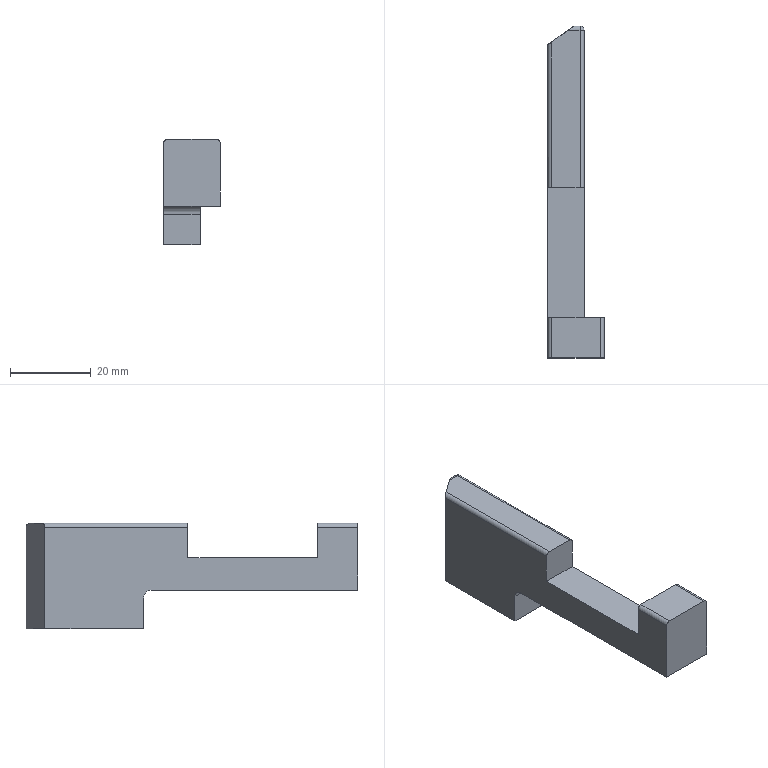Part | NX | features DIE-37 2 | 1 solid | 22 faces | box 14 x 82 x 26 mm | volume 12622 mm3 | plane 14 | cylinder 7 | sphere 1 | commonest cylinder face diameters 2 x6 4 x1
STEP:
#1=CARTESIAN_POINT('',(2459.569,-953.622,868.716));
#2=VERTEX_POINT('',#1);
#3=CARTESIAN_POINT('',(2459.569,-1004.622,868.716));
#4=VERTEX_POINT('',#3);
#5=CARTESIAN_POINT('',(2459.569,-923.622,868.716));
#6=DIRECTION('',(0.,-1.,0.));
#7=VECTOR('',#6,1000.);
#8=LINE('',#5,#7);
#9=EDGE_CURVE('',#2,#4,#8,.T.);
#10=ORIENTED_EDGE('',*,*,#9,.F.);
#11=CARTESIAN_POINT('',(2468.569,-953.622,868.716));
#12=VERTEX_POINT('',#11);
#13=CARTESIAN_POINT('',(2465.569,-953.622,868.716));
#14=DIRECTION('',(1.,0.,0.));
#15=VECTOR('',#14,1000.);
#16=LINE('',#13,#15);
#17=EDGE_CURVE('',#2,#12,#16,.T.);
#18=ORIENTED_EDGE('',*,*,#17,.T.);
#19=CARTESIAN_POINT('',(2468.569,-994.622,868.716));
#20=VERTEX_POINT('',#19);
#21=CARTESIAN_POINT('',(2468.569,-923.622,868.716));
#22=DIRECTION('',(0.,1.,0.));
#23=VECTOR('',#22,1000.);
#24=LINE('',#21,#23);
#25=EDGE_CURVE('',#20,#12,#24,.T.);
#26=ORIENTED_EDGE('',*,*,#25,.F.);
#27=CARTESIAN_POINT('',(2473.569,-994.622,868.716));
#28=VERTEX_POINT('',#27);
#29=CARTESIAN_POINT('',(2465.569,-994.622,868.716));
#30=DIRECTION('',(-1.,0.,0.));
#31=VECTOR('',#30,1000.);
#32=LINE('',#29,#31);
#33=EDGE_CURVE('',#28,#20,#32,.T.);
#34=ORIENTED_EDGE('',*,*,#33,.F.);
#35=CARTESIAN_POINT('',(2473.569,-1004.622,868.716));
#36=VERTEX_POINT('',#35);
#37=CARTESIAN_POINT('',(2473.569,-923.622,868.716));
#38=DIRECTION('',(0.,1.,0.));
#39=VECTOR('',#38,1000.);
#40=LINE('',#37,#39);
#41=EDGE_CURVE('',#36,#28,#40,.T.);
#42=ORIENTED_EDGE('',*,*,#41,.F.);
#43=CARTESIAN_POINT('',(2691.569,-1004.622,868.716));
#44=DIRECTION('',(1.,0.,0.));
#45=VECTOR('',#44,1000.);
#46=LINE('',#43,#45);
#47=EDGE_CURVE('',#4,#36,#46,.T.);
#48=ORIENTED_EDGE('',*,*,#47,.F.);
#49=EDGE_LOOP('',(#10,#18,#26,#34,#42,#48));
#50=FACE_BOUND('',#49,.T.);
#51=CARTESIAN_POINT('',(2465.569,-923.622,868.716));
#52=DIRECTION('',(0.,0.,-1.));
#53=DIRECTION('',(1.,0.,0.));
#54=AXIS2_PLACEMENT_3D('',#51,#52,#53);
#55=PLANE('',#54);
#56=ADVANCED_FACE('',(#50),#55,.T.);
#57=CARTESIAN_POINT('',(2468.569,-994.622,876.716));
#58=VERTEX_POINT('',#57);
#59=CARTESIAN_POINT('',(2468.569,-994.622,868.716));
#60=DIRECTION('',(0.,0.,-1.));
#61=VECTOR('',#60,1000.);
#62=LINE('',#59,#61);
#63=EDGE_CURVE('',#58,#20,#62,.T.);
#64=ORIENTED_EDGE('',*,*,#63,.F.);
#65=CARTESIAN_POINT('',(2459.569,-994.622,876.716));
#66=VERTEX_POINT('',#65);
#67=CARTESIAN_POINT('',(2691.569,-994.622,876.716));
#68=DIRECTION('',(-1.,0.,0.));
#69=VECTOR('',#68,1000.);
#70=LINE('',#67,#69);
#71=EDGE_CURVE('',#58,#66,#70,.T.);
#72=ORIENTED_EDGE('',*,*,#71,.T.);
#73=CARTESIAN_POINT('',(2459.569,-994.622,884.216));
#74=VERTEX_POINT('',#73);
#75=CARTESIAN_POINT('',(2459.569,-994.622,868.716));
#76=DIRECTION('',(0.,0.,1.));
#77=VECTOR('',#76,1000.);
#78=LINE('',#75,#77);
#79=EDGE_CURVE('',#66,#74,#78,.T.);
#80=ORIENTED_EDGE('',*,*,#79,.T.);
#81=CARTESIAN_POINT('',(2460.569,-994.622,885.216));
#82=VERTEX_POINT('',#81);
#83=CARTESIAN_POINT('',(2460.569,-994.622,884.216));
#84=DIRECTION('',(0.,1.,0.));
#85=DIRECTION('',(0.,0.,-1.));
#86=AXIS2_PLACEMENT_3D('',#83,#84,#85);
#87=CIRCLE('',#86,1.);
#88=EDGE_CURVE('',#74,#82,#87,.T.);
#89=ORIENTED_EDGE('',*,*,#88,.T.);
#90=CARTESIAN_POINT('',(2472.569,-994.622,885.216));
#91=VERTEX_POINT('',#90);
#92=CARTESIAN_POINT('',(2691.569,-994.622,885.216));
#93=DIRECTION('',(-1.,0.,0.));
#94=VECTOR('',#93,1000.);
#95=LINE('',#92,#94);
#96=EDGE_CURVE('',#91,#82,#95,.T.);
#97=ORIENTED_EDGE('',*,*,#96,.F.);
#98=CARTESIAN_POINT('',(2473.569,-994.622,884.216));
#99=VERTEX_POINT('',#98);
#100=CARTESIAN_POINT('',(2472.569,-994.622,884.216));
#101=DIRECTION('',(0.,1.,0.));
#102=DIRECTION('',(0.,0.,-1.));
#103=AXIS2_PLACEMENT_3D('',#100,#101,#102);
#104=CIRCLE('',#103,1.);
#105=EDGE_CURVE('',#91,#99,#104,.T.);
#106=ORIENTED_EDGE('',*,*,#105,.T.);
#107=CARTESIAN_POINT('',(2473.569,-994.622,803.716));
#108=DIRECTION('',(0.,0.,1.));
#109=VECTOR('',#108,1000.);
#110=LINE('',#107,#109);
#111=EDGE_CURVE('',#28,#99,#110,.T.);
#112=ORIENTED_EDGE('',*,*,#111,.F.);
#113=ORIENTED_EDGE('',*,*,#33,.T.);
#114=EDGE_LOOP('',(#64,#72,#80,#89,#97,#106,#112,#113));
#115=FACE_BOUND('',#114,.T.);
#116=CARTESIAN_POINT('',(2691.569,-994.622,803.716));
#117=DIRECTION('',(0.,-1.,0.));
#118=DIRECTION('',(0.,0.,-1.));
#119=AXIS2_PLACEMENT_3D('',#116,#117,#118);
#120=PLANE('',#119);
#121=ADVANCED_FACE('',(#115),#120,.F.);
#122=ORIENTED_EDGE('',*,*,#96,.T.);
#123=CARTESIAN_POINT('',(2460.569,-1004.622,885.216));
#124=VERTEX_POINT('',#123);
#125=CARTESIAN_POINT('',(2460.569,-913.622,885.216));
#126=DIRECTION('',(0.,-1.,0.));
#127=VECTOR('',#126,1000.);
#128=LINE('',#125,#127);
#129=EDGE_CURVE('',#82,#124,#128,.T.);
#130=ORIENTED_EDGE('',*,*,#129,.T.);
#131=CARTESIAN_POINT('',(2472.569,-1004.622,885.216));
#132=VERTEX_POINT('',#131);
#133=CARTESIAN_POINT('',(2691.569,-1004.622,885.216));
#134=DIRECTION('',(-1.,0.,0.));
#135=VECTOR('',#134,1000.);
#136=LINE('',#133,#135);
#137=EDGE_CURVE('',#132,#124,#136,.T.);
#138=ORIENTED_EDGE('',*,*,#137,.F.);
#139=CARTESIAN_POINT('',(2472.569,-913.622,885.216));
#140=DIRECTION('',(0.,1.,0.));
#141=VECTOR('',#140,1000.);
#142=LINE('',#139,#141);
#143=EDGE_CURVE('',#132,#91,#142,.T.);
#144=ORIENTED_EDGE('',*,*,#143,.T.);
#145=EDGE_LOOP('',(#122,#130,#138,#144));
#146=FACE_BOUND('',#145,.T.);
#147=CARTESIAN_POINT('',(2465.569,-913.622,885.216));
#148=DIRECTION('',(0.,0.,1.));
#149=DIRECTION('',(-1.,0.,0.));
#150=AXIS2_PLACEMENT_3D('',#147,#148,#149);
#151=PLANE('',#150);
#152=ADVANCED_FACE('',(#146),#151,.T.);
#153=ORIENTED_EDGE('',*,*,#105,.F.);
#154=ORIENTED_EDGE('',*,*,#143,.F.);
#155=CARTESIAN_POINT('',(2473.569,-1004.622,884.216));
#156=VERTEX_POINT('',#155);
#157=CARTESIAN_POINT('',(2472.569,-1004.622,884.216));
#158=DIRECTION('',(0.,-1.,0.));
#159=DIRECTION('',(0.,0.,-1.));
#160=AXIS2_PLACEMENT_3D('',#157,#158,#159);
#161=CIRCLE('',#160,1.);
#162=EDGE_CURVE('',#156,#132,#161,.T.);
#163=ORIENTED_EDGE('',*,*,#162,.F.);
#164=CARTESIAN_POINT('',(2473.569,-913.622,884.216));
#165=DIRECTION('',(0.,-1.,0.));
#166=VECTOR('',#165,1000.);
#167=LINE('',#164,#166);
#168=EDGE_CURVE('',#99,#156,#167,.T.);
#169=ORIENTED_EDGE('',*,*,#168,.F.);
#170=EDGE_LOOP('',(#153,#154,#163,#169));
#171=FACE_BOUND('',#170,.T.);
#172=CARTESIAN_POINT('',(2472.569,-913.622,884.216));
#173=DIRECTION('',(0.,-1.,0.));
#174=DIRECTION('',(0.,0.,1.));
#175=AXIS2_PLACEMENT_3D('',#172,#173,#174);
#176=CYLINDRICAL_SURFACE('',#175,1.);
#177=ADVANCED_FACE('',(#171),#176,.T.);
#178=CARTESIAN_POINT('',(2459.569,-1004.622,884.216));
#179=VERTEX_POINT('',#178);
#180=CARTESIAN_POINT('',(2460.569,-1004.622,884.216));
#181=DIRECTION('',(0.,-1.,0.));
#182=DIRECTION('',(0.,0.,-1.));
#183=AXIS2_PLACEMENT_3D('',#180,#181,#182);
#184=CIRCLE('',#183,1.);
#185=EDGE_CURVE('',#124,#179,#184,.T.);
#186=ORIENTED_EDGE('',*,*,#185,.F.);
#187=ORIENTED_EDGE('',*,*,#129,.F.);
#188=ORIENTED_EDGE('',*,*,#88,.F.);
#189=CARTESIAN_POINT('',(2459.569,-913.622,884.216));
#190=DIRECTION('',(0.,1.,0.));
#191=VECTOR('',#190,1000.);
#192=LINE('',#189,#191);
#193=EDGE_CURVE('',#179,#74,#192,.T.);
#194=ORIENTED_EDGE('',*,*,#193,.F.);
#195=EDGE_LOOP('',(#186,#187,#188,#194));
#196=FACE_BOUND('',#195,.T.);
#197=CARTESIAN_POINT('',(2460.569,-913.622,884.216));
#198=DIRECTION('',(0.,1.,0.));
#199=DIRECTION('',(0.,0.,-1.));
#200=AXIS2_PLACEMENT_3D('',#197,#198,#199);
#201=CYLINDRICAL_SURFACE('',#200,1.);
#202=ADVANCED_FACE('',(#196),#201,.T.);
#203=ORIENTED_EDGE('',*,*,#137,.T.);
#204=ORIENTED_EDGE('',*,*,#185,.T.);
#205=CARTESIAN_POINT('',(2459.569,-1004.622,868.716));
#206=DIRECTION('',(0.,0.,1.));
#207=VECTOR('',#206,1000.);
#208=LINE('',#205,#207);
#209=EDGE_CURVE('',#4,#179,#208,.T.);
#210=ORIENTED_EDGE('',*,*,#209,.F.);
#211=ORIENTED_EDGE('',*,*,#47,.T.);
#212=CARTESIAN_POINT('',(2473.569,-1004.622,803.716));
#213=DIRECTION('',(0.,0.,1.));
#214=VECTOR('',#213,1000.);
#215=LINE('',#212,#214);
#216=EDGE_CURVE('',#36,#156,#215,.T.);
#217=ORIENTED_EDGE('',*,*,#216,.T.);
#218=ORIENTED_EDGE('',*,*,#162,.T.);
#219=EDGE_LOOP('',(#203,#204,#210,#211,#217,#218));
#220=FACE_BOUND('',#219,.T.);
#221=CARTESIAN_POINT('',(2691.569,-1004.622,803.716));
#222=DIRECTION('',(0.,-1.,0.));
#223=DIRECTION('',(0.,0.,-1.));
#224=AXIS2_PLACEMENT_3D('',#221,#222,#223);
#225=PLANE('',#224);
#226=ADVANCED_FACE('',(#220),#225,.T.);
#227=ORIENTED_EDGE('',*,*,#79,.F.);
#228=CARTESIAN_POINT('',(2459.569,-962.622,876.716));
#229=VERTEX_POINT('',#228);
#230=CARTESIAN_POINT('',(2459.569,-923.622,876.716));
#231=DIRECTION('',(0.,1.,0.));
#232=VECTOR('',#231,1000.);
#233=LINE('',#230,#232);
#234=EDGE_CURVE('',#66,#229,#233,.T.);
#235=ORIENTED_EDGE('',*,*,#234,.T.);
#236=CARTESIAN_POINT('',(2459.569,-962.622,884.216));
#237=VERTEX_POINT('',#236);
#238=CARTESIAN_POINT('',(2459.569,-962.622,868.716));
#239=DIRECTION('',(0.,0.,-1.));
#240=VECTOR('',#239,1000.);
#241=LINE('',#238,#240);
#242=EDGE_CURVE('',#237,#229,#241,.T.);
#243=ORIENTED_EDGE('',*,*,#242,.F.);
#244=CARTESIAN_POINT('',(2459.569,-927.265,884.216));
#245=VERTEX_POINT('',#244);
#246=CARTESIAN_POINT('',(2459.569,-923.622,884.216));
#247=DIRECTION('',(0.,1.,0.));
#248=VECTOR('',#247,1000.);
#249=LINE('',#246,#248);
#250=EDGE_CURVE('',#237,#245,#249,.T.);
#251=ORIENTED_EDGE('',*,*,#250,.T.);
#252=CARTESIAN_POINT('',(2459.569,-927.265,859.216));
#253=VERTEX_POINT('',#252);
#254=CARTESIAN_POINT('',(2459.569,-927.265,868.716));
#255=DIRECTION('',(0.,0.,-1.));
#256=VECTOR('',#255,1000.);
#257=LINE('',#254,#256);
#258=EDGE_CURVE('',#245,#253,#257,.T.);
#259=ORIENTED_EDGE('',*,*,#258,.T.);
#260=CARTESIAN_POINT('',(2459.569,-951.622,859.216));
#261=VERTEX_POINT('',#260);
#262=CARTESIAN_POINT('',(2459.569,-923.622,859.216));
#263=DIRECTION('',(0.,-1.,0.));
#264=VECTOR('',#263,1000.);
#265=LINE('',#262,#264);
#266=EDGE_CURVE('',#253,#261,#265,.T.);
#267=ORIENTED_EDGE('',*,*,#266,.T.);
#268=CARTESIAN_POINT('',(2459.569,-951.622,866.716));
#269=VERTEX_POINT('',#268);
#270=CARTESIAN_POINT('',(2459.569,-951.622,868.716));
#271=DIRECTION('',(0.,0.,1.));
#272=VECTOR('',#271,1000.);
#273=LINE('',#270,#272);
#274=EDGE_CURVE('',#261,#269,#273,.T.);
#275=ORIENTED_EDGE('',*,*,#274,.T.);
#276=CARTESIAN_POINT('',(2459.569,-953.622,866.716));
#277=DIRECTION('',(-1.,0.,0.));
#278=DIRECTION('',(0.,0.,1.));
#279=AXIS2_PLACEMENT_3D('',#276,#277,#278);
#280=CIRCLE('',#279,2.);
#281=EDGE_CURVE('',#269,#2,#280,.F.);
#282=ORIENTED_EDGE('',*,*,#281,.T.);
#283=ORIENTED_EDGE('',*,*,#9,.T.);
#284=ORIENTED_EDGE('',*,*,#209,.T.);
#285=ORIENTED_EDGE('',*,*,#193,.T.);
#286=EDGE_LOOP('',(#227,#235,#243,#251,#259,#267,#275,#282,#283,#284,#285));
#287=FACE_BOUND('',#286,.T.);
#288=CARTESIAN_POINT('',(2459.569,-923.622,868.716));
#289=DIRECTION('',(-1.,0.,0.));
#290=DIRECTION('',(0.,0.,-1.));
#291=AXIS2_PLACEMENT_3D('',#288,#289,#290);
#292=PLANE('',#291);
#293=ADVANCED_FACE('',(#287),#292,.T.);
#294=ORIENTED_EDGE('',*,*,#41,.T.);
#295=ORIENTED_EDGE('',*,*,#111,.T.);
#296=ORIENTED_EDGE('',*,*,#168,.T.);
#297=ORIENTED_EDGE('',*,*,#216,.F.);
#298=EDGE_LOOP('',(#294,#295,#296,#297));
#299=FACE_BOUND('',#298,.T.);
#300=CARTESIAN_POINT('',(2473.569,-923.622,868.716));
#301=DIRECTION('',(1.,0.,0.));
#302=DIRECTION('',(0.,0.,1.));
#303=AXIS2_PLACEMENT_3D('',#300,#301,#302);
#304=PLANE('',#303);
#305=ADVANCED_FACE('',(#299),#304,.T.);
#306=ORIENTED_EDGE('',*,*,#25,.T.);
#307=CARTESIAN_POINT('',(2468.569,-951.622,866.716));
#308=VERTEX_POINT('',#307);
#309=CARTESIAN_POINT('',(2468.569,-953.622,866.716));
#310=DIRECTION('',(1.,0.,0.));
#311=DIRECTION('',(0.,0.,-1.));
#312=AXIS2_PLACEMENT_3D('',#309,#310,#311);
#313=CIRCLE('',#312,2.);
#314=EDGE_CURVE('',#12,#308,#313,.F.);
#315=ORIENTED_EDGE('',*,*,#314,.T.);
#316=CARTESIAN_POINT('',(2468.569,-951.622,859.216));
#317=VERTEX_POINT('',#316);
#318=CARTESIAN_POINT('',(2468.569,-951.622,868.716));
#319=DIRECTION('',(0.,0.,-1.));
#320=VECTOR('',#319,1000.);
#321=LINE('',#318,#320);
#322=EDGE_CURVE('',#317,#308,#321,.F.);
#323=ORIENTED_EDGE('',*,*,#322,.F.);
#324=CARTESIAN_POINT('',(2468.569,-923.622,859.216));
#325=VERTEX_POINT('',#324);
#326=CARTESIAN_POINT('',(2468.569,-923.622,859.216));
#327=DIRECTION('',(0.,1.,0.));
#328=VECTOR('',#327,1000.);
#329=LINE('',#326,#328);
#330=EDGE_CURVE('',#317,#325,#329,.T.);
#331=ORIENTED_EDGE('',*,*,#330,.T.);
#332=CARTESIAN_POINT('',(2468.569,-923.622,884.216));
#333=VERTEX_POINT('',#332);
#334=CARTESIAN_POINT('',(2468.569,-923.622,868.716));
#335=DIRECTION('',(0.,0.,1.));
#336=VECTOR('',#335,1000.);
#337=LINE('',#334,#336);
#338=EDGE_CURVE('',#325,#333,#337,.T.);
#339=ORIENTED_EDGE('',*,*,#338,.T.);
#340=CARTESIAN_POINT('',(2468.569,-962.622,884.216));
#341=VERTEX_POINT('',#340);
#342=CARTESIAN_POINT('',(2468.569,-923.622,884.216));
#343=DIRECTION('',(0.,-1.,0.));
#344=VECTOR('',#343,1000.);
#345=LINE('',#342,#344);
#346=EDGE_CURVE('',#333,#341,#345,.T.);
#347=ORIENTED_EDGE('',*,*,#346,.T.);
#348=CARTESIAN_POINT('',(2468.569,-962.622,876.716));
#349=VERTEX_POINT('',#348);
#350=CARTESIAN_POINT('',(2468.569,-962.622,868.716));
#351=DIRECTION('',(0.,0.,1.));
#352=VECTOR('',#351,1000.);
#353=LINE('',#350,#352);
#354=EDGE_CURVE('',#349,#341,#353,.T.);
#355=ORIENTED_EDGE('',*,*,#354,.F.);
#356=CARTESIAN_POINT('',(2468.569,-923.622,876.716));
#357=DIRECTION('',(0.,-1.,0.));
#358=VECTOR('',#357,1000.);
#359=LINE('',#356,#358);
#360=EDGE_CURVE('',#349,#58,#359,.T.);
#361=ORIENTED_EDGE('',*,*,#360,.T.);
#362=ORIENTED_EDGE('',*,*,#63,.T.);
#363=EDGE_LOOP('',(#306,#315,#323,#331,#339,#347,#355,#361,#362));
#364=FACE_BOUND('',#363,.T.);
#365=CARTESIAN_POINT('',(2468.569,-923.622,868.716));
#366=DIRECTION('',(1.,0.,0.));
#367=DIRECTION('',(0.,0.,1.));
#368=AXIS2_PLACEMENT_3D('',#365,#366,#367);
#369=PLANE('',#368);
#370=ADVANCED_FACE('',(#364),#369,.T.);
#371=ORIENTED_EDGE('',*,*,#234,.F.);
#372=ORIENTED_EDGE('',*,*,#71,.F.);
#373=ORIENTED_EDGE('',*,*,#360,.F.);
#374=CARTESIAN_POINT('',(2463.569,-962.622,876.716));
#375=DIRECTION('',(-1.,0.,0.));
#376=VECTOR('',#375,1000.);
#377=LINE('',#374,#376);
#378=EDGE_CURVE('',#349,#229,#377,.T.);
#379=ORIENTED_EDGE('',*,*,#378,.T.);
#380=EDGE_LOOP('',(#371,#372,#373,#379));
#381=FACE_BOUND('',#380,.T.);
#382=CARTESIAN_POINT('',(2463.569,-948.622,876.716));
#383=DIRECTION('',(0.,0.,1.));
#384=DIRECTION('',(-1.,0.,0.));
#385=AXIS2_PLACEMENT_3D('',#382,#383,#384);
#386=PLANE('',#385);
#387=ADVANCED_FACE('',(#381),#386,.T.);
#388=CARTESIAN_POINT('',(2466.069,-922.622,884.216));
#389=VERTEX_POINT('',#388);
#390=CARTESIAN_POINT('',(2467.569,-922.622,884.216));
#391=VERTEX_POINT('',#390);
#392=CARTESIAN_POINT('',(2465.569,-922.622,884.216));
#393=DIRECTION('',(1.,0.,0.));
#394=VECTOR('',#393,1000.);
#395=LINE('',#392,#394);
#396=EDGE_CURVE('',#389,#391,#395,.T.);
#397=ORIENTED_EDGE('',*,*,#396,.T.);
#398=CARTESIAN_POINT('',(2467.569,-922.622,859.216));
#399=VERTEX_POINT('',#398);
#400=CARTESIAN_POINT('',(2467.569,-922.622,868.716));
#401=DIRECTION('',(0.,0.,1.));
#402=VECTOR('',#401,1000.);
#403=LINE('',#400,#402);
#404=EDGE_CURVE('',#391,#399,#403,.F.);
#405=ORIENTED_EDGE('',*,*,#404,.T.);
#406=CARTESIAN_POINT('',(2466.069,-922.622,859.216));
#407=VERTEX_POINT('',#406);
#408=CARTESIAN_POINT('',(2465.569,-922.622,859.216));
#409=DIRECTION('',(-1.,0.,0.));
#410=VECTOR('',#409,1000.);
#411=LINE('',#408,#410);
#412=EDGE_CURVE('',#399,#407,#411,.T.);
#413=ORIENTED_EDGE('',*,*,#412,.T.);
#414=CARTESIAN_POINT('',(2466.069,-922.622,868.716));
#415=DIRECTION('',(0.,0.,1.));
#416=VECTOR('',#415,1000.);
#417=LINE('',#414,#416);
#418=EDGE_CURVE('',#407,#389,#417,.T.);
#419=ORIENTED_EDGE('',*,*,#418,.T.);
#420=EDGE_LOOP('',(#397,#405,#413,#419));
#421=FACE_BOUND('',#420,.T.);
#422=CARTESIAN_POINT('',(2465.569,-922.622,868.716));
#423=DIRECTION('',(0.,1.,0.));
#424=DIRECTION('',(0.,0.,-1.));
#425=AXIS2_PLACEMENT_3D('',#422,#423,#424);
#426=PLANE('',#425);
#427=ADVANCED_FACE('',(#421),#426,.T.);
#428=ORIENTED_EDGE('',*,*,#258,.F.);
#429=CARTESIAN_POINT('',(2460.569,-926.551,885.216));
#430=VERTEX_POINT('',#429);
#431=CARTESIAN_POINT('',(2460.569,-926.551,884.216));
#432=DIRECTION('',(-0.5812,0.8137,0.));
#433=DIRECTION('',(0.8137,0.5812,0.));
#434=AXIS2_PLACEMENT_3D('',#431,#432,#433);
#435=ELLIPSE('',#434,1.229,1.);
#436=EDGE_CURVE('',#245,#430,#435,.T.);
#437=ORIENTED_EDGE('',*,*,#436,.T.);
#438=CARTESIAN_POINT('',(2464.669,-923.622,885.216));
#439=VERTEX_POINT('',#438);
#440=CARTESIAN_POINT('',(2465.265,-923.196,885.216));
#441=DIRECTION('',(-0.8137,-0.5812,0.));
#442=VECTOR('',#441,1000.);
#443=LINE('',#440,#442);
#444=EDGE_CURVE('',#439,#430,#443,.T.);
#445=ORIENTED_EDGE('',*,*,#444,.F.);
#446=CARTESIAN_POINT('',(2464.669,-923.622,884.216));
#447=DIRECTION('',(-0.5812,0.8137,0.));
#448=DIRECTION('',(0.8137,0.5812,0.));
#449=AXIS2_PLACEMENT_3D('',#446,#447,#448);
#450=ELLIPSE('',#449,1.72,1.);
#451=EDGE_CURVE('',#439,#389,#450,.T.);
#452=ORIENTED_EDGE('',*,*,#451,.T.);
#453=ORIENTED_EDGE('',*,*,#418,.F.);
#454=CARTESIAN_POINT('',(2466.069,-922.622,859.216));
#455=DIRECTION('',(0.8137,0.5812,0.));
#456=VECTOR('',#455,1000.);
#457=LINE('',#454,#456);
#458=EDGE_CURVE('',#253,#407,#457,.T.);
#459=ORIENTED_EDGE('',*,*,#458,.F.);
#460=EDGE_LOOP('',(#428,#437,#445,#452,#453,#459));
#461=FACE_BOUND('',#460,.T.);
#462=CARTESIAN_POINT('',(2466.069,-922.622,868.716));
#463=DIRECTION('',(0.5812,-0.8137,0.));
#464=DIRECTION('',(0.,0.,-1.));
#465=AXIS2_PLACEMENT_3D('',#462,#463,#464);
#466=PLANE('',#465);
#467=ADVANCED_FACE('',(#461),#466,.F.);
#468=ORIENTED_EDGE('',*,*,#444,.T.);
#469=CARTESIAN_POINT('',(2460.569,-962.622,885.216));
#470=VERTEX_POINT('',#469);
#471=CARTESIAN_POINT('',(2460.569,-923.622,885.216));
#472=DIRECTION('',(0.,-1.,0.));
#473=VECTOR('',#472,1000.);
#474=LINE('',#471,#473);
#475=EDGE_CURVE('',#430,#470,#474,.T.);
#476=ORIENTED_EDGE('',*,*,#475,.T.);
#477=CARTESIAN_POINT('',(2467.569,-962.622,885.216));
#478=VERTEX_POINT('',#477);
#479=CARTESIAN_POINT('',(2463.569,-962.622,885.216));
#480=DIRECTION('',(1.,0.,0.));
#481=VECTOR('',#480,1000.);
#482=LINE('',#479,#481);
#483=EDGE_CURVE('',#470,#478,#482,.T.);
#484=ORIENTED_EDGE('',*,*,#483,.T.);
#485=CARTESIAN_POINT('',(2467.569,-923.622,885.216));
#486=VERTEX_POINT('',#485);
#487=CARTESIAN_POINT('',(2467.569,-923.622,885.216));
#488=DIRECTION('',(0.,1.,0.));
#489=VECTOR('',#488,1000.);
#490=LINE('',#487,#489);
#491=EDGE_CURVE('',#478,#486,#490,.T.);
#492=ORIENTED_EDGE('',*,*,#491,.T.);
#493=CARTESIAN_POINT('',(2465.569,-923.622,885.216));
#494=DIRECTION('',(-1.,0.,0.));
#495=VECTOR('',#494,1000.);
#496=LINE('',#493,#495);
#497=EDGE_CURVE('',#486,#439,#496,.T.);
#498=ORIENTED_EDGE('',*,*,#497,.T.);
#499=EDGE_LOOP('',(#468,#476,#484,#492,#498));
#500=FACE_BOUND('',#499,.T.);
#501=CARTESIAN_POINT('',(2465.569,-923.622,885.216));
#502=DIRECTION('',(0.,0.,1.));
#503=DIRECTION('',(-1.,0.,0.));
#504=AXIS2_PLACEMENT_3D('',#501,#502,#503);
#505=PLANE('',#504);
#506=ADVANCED_FACE('',(#500),#505,.T.);
#507=ORIENTED_EDGE('',*,*,#483,.F.);
#508=CARTESIAN_POINT('',(2460.569,-962.622,884.216));
#509=DIRECTION('',(0.,-1.,0.));
#510=DIRECTION('',(0.,0.,1.));
#511=AXIS2_PLACEMENT_3D('',#508,#509,#510);
#512=CIRCLE('',#511,1.);
#513=EDGE_CURVE('',#470,#237,#512,.T.);
#514=ORIENTED_EDGE('',*,*,#513,.T.);
#515=ORIENTED_EDGE('',*,*,#242,.T.);
#516=ORIENTED_EDGE('',*,*,#378,.F.);
#517=ORIENTED_EDGE('',*,*,#354,.T.);
#518=CARTESIAN_POINT('',(2467.569,-962.622,884.216));
#519=DIRECTION('',(0.,-1.,0.));
#520=DIRECTION('',(0.,0.,1.));
#521=AXIS2_PLACEMENT_3D('',#518,#519,#520);
#522=CIRCLE('',#521,1.);
#523=EDGE_CURVE('',#341,#478,#522,.T.);
#524=ORIENTED_EDGE('',*,*,#523,.T.);
#525=EDGE_LOOP('',(#507,#514,#515,#516,#517,#524));
#526=FACE_BOUND('',#525,.T.);
#527=CARTESIAN_POINT('',(2463.569,-962.622,860.716));
#528=DIRECTION('',(0.,1.,0.));
#529=DIRECTION('',(0.,0.,-1.));
#530=AXIS2_PLACEMENT_3D('',#527,#528,#529);
#531=PLANE('',#530);
#532=ADVANCED_FACE('',(#526),#531,.F.);
#533=ORIENTED_EDGE('',*,*,#513,.F.);
#534=ORIENTED_EDGE('',*,*,#475,.F.);
#535=ORIENTED_EDGE('',*,*,#436,.F.);
#536=ORIENTED_EDGE('',*,*,#250,.F.);
#537=EDGE_LOOP('',(#533,#534,#535,#536));
#538=FACE_BOUND('',#537,.T.);
#539=CARTESIAN_POINT('',(2460.569,-923.622,884.216));
#540=DIRECTION('',(0.,1.,0.));
#541=DIRECTION('',(0.,0.,-1.));
#542=AXIS2_PLACEMENT_3D('',#539,#540,#541);
#543=CYLINDRICAL_SURFACE('',#542,1.);
#544=ADVANCED_FACE('',(#538),#543,.T.);
#545=ORIENTED_EDGE('',*,*,#346,.F.);
#546=CARTESIAN_POINT('',(2467.569,-923.622,884.216));
#547=DIRECTION('',(0.,-1.,0.));
#548=DIRECTION('',(0.,0.,-1.));
#549=AXIS2_PLACEMENT_3D('',#546,#547,#548);
#550=CIRCLE('',#549,1.);
#551=EDGE_CURVE('',#333,#486,#550,.T.);
#552=ORIENTED_EDGE('',*,*,#551,.T.);
#553=ORIENTED_EDGE('',*,*,#491,.F.);
#554=ORIENTED_EDGE('',*,*,#523,.F.);
#555=EDGE_LOOP('',(#545,#552,#553,#554));
#556=FACE_BOUND('',#555,.T.);
#557=CARTESIAN_POINT('',(2467.569,-923.622,884.216));
#558=DIRECTION('',(0.,-1.,0.));
#559=DIRECTION('',(0.,0.,1.));
#560=AXIS2_PLACEMENT_3D('',#557,#558,#559);
#561=CYLINDRICAL_SURFACE('',#560,1.);
#562=ADVANCED_FACE('',(#556),#561,.T.);
#563=ORIENTED_EDGE('',*,*,#497,.F.);
#564=CARTESIAN_POINT('',(2467.569,-923.622,884.216));
#565=DIRECTION('',(1.,0.,0.));
#566=DIRECTION('',(0.,0.,-1.));
#567=AXIS2_PLACEMENT_3D('',#564,#565,#566);
#568=CIRCLE('',#567,1.);
#569=EDGE_CURVE('',#486,#391,#568,.F.);
#570=ORIENTED_EDGE('',*,*,#569,.T.);
#571=ORIENTED_EDGE('',*,*,#396,.F.);
#572=ORIENTED_EDGE('',*,*,#451,.F.);
#573=EDGE_LOOP('',(#563,#570,#571,#572));
#574=FACE_BOUND('',#573,.T.);
#575=CARTESIAN_POINT('',(2465.569,-923.622,884.216));
#576=DIRECTION('',(1.,0.,0.));
#577=DIRECTION('',(0.,0.,1.));
#578=AXIS2_PLACEMENT_3D('',#575,#576,#577);
#579=CYLINDRICAL_SURFACE('',#578,1.);
#580=ADVANCED_FACE('',(#574),#579,.T.);
#581=ORIENTED_EDGE('',*,*,#338,.F.);
#582=CARTESIAN_POINT('',(2467.569,-923.622,859.216));
#583=DIRECTION('',(0.,0.,-1.));
#584=DIRECTION('',(-1.,0.,0.));
#585=AXIS2_PLACEMENT_3D('',#582,#583,#584);
#586=CIRCLE('',#585,1.);
#587=EDGE_CURVE('',#399,#325,#586,.T.);
#588=ORIENTED_EDGE('',*,*,#587,.F.);
#589=ORIENTED_EDGE('',*,*,#404,.F.);
#590=CARTESIAN_POINT('',(2467.569,-923.622,884.216));
#591=DIRECTION('',(0.,0.,1.));
#592=DIRECTION('',(1.,0.,0.));
#593=AXIS2_PLACEMENT_3D('',#590,#591,#592);
#594=CIRCLE('',#593,1.);
#595=EDGE_CURVE('',#333,#391,#594,.T.);
#596=ORIENTED_EDGE('',*,*,#595,.F.);
#597=EDGE_LOOP('',(#581,#588,#589,#596));
#598=FACE_BOUND('',#597,.T.);
#599=CARTESIAN_POINT('',(2467.569,-923.622,868.716));
#600=DIRECTION('',(0.,0.,1.));
#601=DIRECTION('',(1.,0.,0.));
#602=AXIS2_PLACEMENT_3D('',#599,#600,#601);
#603=CYLINDRICAL_SURFACE('',#602,1.);
#604=ADVANCED_FACE('',(#598),#603,.T.);
#605=ORIENTED_EDGE('',*,*,#569,.F.);
#606=ORIENTED_EDGE('',*,*,#551,.F.);
#607=ORIENTED_EDGE('',*,*,#595,.T.);
#608=EDGE_LOOP('',(#605,#606,#607));
#609=FACE_BOUND('',#608,.T.);
#610=CARTESIAN_POINT('',(2467.569,-923.622,884.216));
#611=DIRECTION('',(0.,0.,1.));
#612=DIRECTION('',(1.,0.,0.));
#613=AXIS2_PLACEMENT_3D('',#610,#611,#612);
#614=SPHERICAL_SURFACE('',#613,1.);
#615=ADVANCED_FACE('',(#609),#614,.T.);
#616=CARTESIAN_POINT('',(2465.569,-951.622,859.216));
#617=DIRECTION('',(1.,0.,0.));
#618=VECTOR('',#617,1000.);
#619=LINE('',#616,#618);
#620=EDGE_CURVE('',#261,#317,#619,.T.);
#621=ORIENTED_EDGE('',*,*,#620,.F.);
#622=ORIENTED_EDGE('',*,*,#266,.F.);
#623=ORIENTED_EDGE('',*,*,#458,.T.);
#624=ORIENTED_EDGE('',*,*,#412,.F.);
#625=ORIENTED_EDGE('',*,*,#587,.T.);
#626=ORIENTED_EDGE('',*,*,#330,.F.);
#627=EDGE_LOOP('',(#621,#622,#623,#624,#625,#626));
#628=FACE_BOUND('',#627,.T.);
#629=CARTESIAN_POINT('',(2465.569,-923.622,859.216));
#630=DIRECTION('',(0.,0.,-1.));
#631=DIRECTION('',(1.,0.,0.));
#632=AXIS2_PLACEMENT_3D('',#629,#630,#631);
#633=PLANE('',#632);
#634=ADVANCED_FACE('',(#628),#633,.T.);
#635=ORIENTED_EDGE('',*,*,#322,.T.);
#636=CARTESIAN_POINT('',(2464.069,-951.622,866.716));
#637=DIRECTION('',(1.,0.,0.));
#638=VECTOR('',#637,1000.);
#639=LINE('',#636,#638);
#640=EDGE_CURVE('',#308,#269,#639,.F.);
#641=ORIENTED_EDGE('',*,*,#640,.T.);
#642=ORIENTED_EDGE('',*,*,#274,.F.);
#643=ORIENTED_EDGE('',*,*,#620,.T.);
#644=EDGE_LOOP('',(#635,#641,#642,#643));
#645=FACE_BOUND('',#644,.T.);
#646=CARTESIAN_POINT('',(2464.069,-951.622,878.466));
#647=DIRECTION('',(0.,1.,0.));
#648=DIRECTION('',(0.,0.,1.));
#649=AXIS2_PLACEMENT_3D('',#646,#647,#648);
#650=PLANE('',#649);
#651=ADVANCED_FACE('',(#645),#650,.F.);
#652=ORIENTED_EDGE('',*,*,#281,.F.);
#653=ORIENTED_EDGE('',*,*,#640,.F.);
#654=ORIENTED_EDGE('',*,*,#314,.F.);
#655=ORIENTED_EDGE('',*,*,#17,.F.);
#656=EDGE_LOOP('',(#652,#653,#654,#655));
#657=FACE_BOUND('',#656,.T.);
#658=CARTESIAN_POINT('',(2465.569,-953.622,866.716));
#659=DIRECTION('',(1.,0.,0.));
#660=DIRECTION('',(0.,0.,-1.));
#661=AXIS2_PLACEMENT_3D('',#658,#659,#660);
#662=CYLINDRICAL_SURFACE('',#661,2.);
#663=ADVANCED_FACE('',(#657),#662,.F.);
#664=CLOSED_SHELL('',(#56,#121,#152,#177,#202,#226,#293,#305,#370,#387,#427,#467,#506,#532,#544,#562,#580,#604,#615,#634,#651,#663));
#665=MANIFOLD_SOLID_BREP('',#664);
#666=(LENGTH_UNIT()NAMED_UNIT(*)SI_UNIT(.MILLI.,.METRE.));
#667=UNCERTAINTY_MEASURE_WITH_UNIT(LENGTH_MEASURE(0.00001),#666,'','');
#668=(NAMED_UNIT(*)PLANE_ANGLE_UNIT()SI_UNIT($,.RADIAN.));
#669=(NAMED_UNIT(*)SI_UNIT($,.STERADIAN.)SOLID_ANGLE_UNIT());
#670=(GEOMETRIC_REPRESENTATION_CONTEXT(3)GLOBAL_UNCERTAINTY_ASSIGNED_CONTEXT((#667))GLOBAL_UNIT_ASSIGNED_CONTEXT((#666,#668,#669))REPRESENTATION_CONTEXT('',''));
#671=ADVANCED_BREP_SHAPE_REPRESENTATION('',(#665),#670);